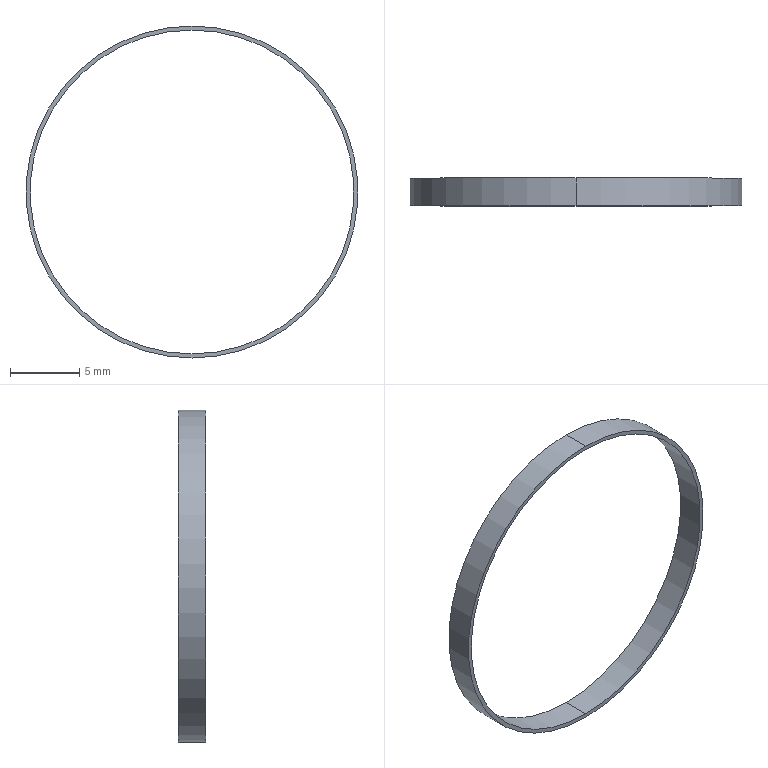Part | SolidWorks | features BaseBody 1 | 1 solid | 6 faces | box 24 x 2 x 24 mm | volume 44.673 mm3 | cylinder 4 | plane 2 | commonest cylinder face diameters 23.4 x2 24 x2
STEP:
#1=CARTESIAN_POINT('',(0.,-1.,12.));
#2=VERTEX_POINT('',#1);
#3=CARTESIAN_POINT('',(0.,-1.,-12.));
#4=VERTEX_POINT('',#3);
#5=CARTESIAN_POINT('',(0.,-1.,0.));
#6=DIRECTION('',(0.,1.,0.));
#7=DIRECTION('',(0.,0.,1.));
#8=AXIS2_PLACEMENT_3D('',#5,#6,#7);
#9=CIRCLE('',#8,12.);
#10=EDGE_CURVE('',#2,#4,#9,.T.);
#11=ORIENTED_EDGE('',*,*,#10,.T.);
#12=CARTESIAN_POINT('',(0.,1.,-12.));
#13=VERTEX_POINT('',#12);
#14=CARTESIAN_POINT('',(0.,-1.,-12.));
#15=DIRECTION('',(0.,1.,0.));
#16=VECTOR('',#15,1000.);
#17=LINE('',#14,#16);
#18=EDGE_CURVE('',#4,#13,#17,.T.);
#19=ORIENTED_EDGE('',*,*,#18,.T.);
#20=CARTESIAN_POINT('',(0.,1.,12.));
#21=VERTEX_POINT('',#20);
#22=CARTESIAN_POINT('',(0.,1.,0.));
#23=DIRECTION('',(0.,-1.,0.));
#24=DIRECTION('',(0.,0.,1.));
#25=AXIS2_PLACEMENT_3D('',#22,#23,#24);
#26=CIRCLE('',#25,12.);
#27=EDGE_CURVE('',#13,#21,#26,.T.);
#28=ORIENTED_EDGE('',*,*,#27,.T.);
#29=CARTESIAN_POINT('',(0.,-1.,12.));
#30=DIRECTION('',(0.,1.,0.));
#31=VECTOR('',#30,1000.);
#32=LINE('',#29,#31);
#33=EDGE_CURVE('',#2,#21,#32,.T.);
#34=ORIENTED_EDGE('',*,*,#33,.F.);
#35=EDGE_LOOP('',(#11,#19,#28,#34));
#36=FACE_OUTER_BOUND('',#35,.T.);
#37=CARTESIAN_POINT('',(0.,-1.,0.));
#38=DIRECTION('',(0.,1.,0.));
#39=DIRECTION('',(0.,0.,1.));
#40=AXIS2_PLACEMENT_3D('',#37,#38,#39);
#41=CYLINDRICAL_SURFACE('',#40,12.);
#42=ADVANCED_FACE('',(#36),#41,.T.);
#43=CARTESIAN_POINT('',(0.,-1.,11.7));
#44=VERTEX_POINT('',#43);
#45=CARTESIAN_POINT('',(0.,-1.,-11.7));
#46=VERTEX_POINT('',#45);
#47=CARTESIAN_POINT('',(0.,-1.,0.));
#48=DIRECTION('',(0.,-1.,0.));
#49=DIRECTION('',(0.,0.,1.));
#50=AXIS2_PLACEMENT_3D('',#47,#48,#49);
#51=CIRCLE('',#50,11.7);
#52=EDGE_CURVE('',#44,#46,#51,.T.);
#53=ORIENTED_EDGE('',*,*,#52,.T.);
#54=CARTESIAN_POINT('',(0.,1.,-11.7));
#55=VERTEX_POINT('',#54);
#56=CARTESIAN_POINT('',(0.,-2.,-11.7));
#57=DIRECTION('',(0.,1.,0.));
#58=VECTOR('',#57,1000.);
#59=LINE('',#56,#58);
#60=EDGE_CURVE('',#46,#55,#59,.T.);
#61=ORIENTED_EDGE('',*,*,#60,.T.);
#62=CARTESIAN_POINT('',(0.,1.,11.7));
#63=VERTEX_POINT('',#62);
#64=CARTESIAN_POINT('',(0.,1.,0.));
#65=DIRECTION('',(0.,-1.,0.));
#66=DIRECTION('',(0.,0.,1.));
#67=AXIS2_PLACEMENT_3D('',#64,#65,#66);
#68=CIRCLE('',#67,11.7);
#69=EDGE_CURVE('',#63,#55,#68,.T.);
#70=ORIENTED_EDGE('',*,*,#69,.F.);
#71=CARTESIAN_POINT('',(0.,-2.,11.7));
#72=DIRECTION('',(0.,1.,0.));
#73=VECTOR('',#72,1000.);
#74=LINE('',#71,#73);
#75=EDGE_CURVE('',#44,#63,#74,.T.);
#76=ORIENTED_EDGE('',*,*,#75,.F.);
#77=EDGE_LOOP('',(#53,#61,#70,#76));
#78=FACE_OUTER_BOUND('',#77,.T.);
#79=CARTESIAN_POINT('',(0.,-2.,0.));
#80=DIRECTION('',(0.,1.,0.));
#81=DIRECTION('',(0.,0.,1.));
#82=AXIS2_PLACEMENT_3D('',#79,#80,#81);
#83=CYLINDRICAL_SURFACE('',#82,11.7);
#84=ADVANCED_FACE('',(#78),#83,.F.);
#85=ORIENTED_EDGE('',*,*,#18,.F.);
#86=CARTESIAN_POINT('',(0.,-1.,0.));
#87=DIRECTION('',(0.,1.,0.));
#88=DIRECTION('',(0.,0.,1.));
#89=AXIS2_PLACEMENT_3D('',#86,#87,#88);
#90=CIRCLE('',#89,12.);
#91=EDGE_CURVE('',#4,#2,#90,.T.);
#92=ORIENTED_EDGE('',*,*,#91,.T.);
#93=ORIENTED_EDGE('',*,*,#33,.T.);
#94=CARTESIAN_POINT('',(0.,1.,0.));
#95=DIRECTION('',(0.,-1.,0.));
#96=DIRECTION('',(0.,0.,1.));
#97=AXIS2_PLACEMENT_3D('',#94,#95,#96);
#98=CIRCLE('',#97,12.);
#99=EDGE_CURVE('',#21,#13,#98,.T.);
#100=ORIENTED_EDGE('',*,*,#99,.T.);
#101=EDGE_LOOP('',(#85,#92,#93,#100));
#102=FACE_OUTER_BOUND('',#101,.T.);
#103=CARTESIAN_POINT('',(0.,-1.,0.));
#104=DIRECTION('',(0.,1.,0.));
#105=DIRECTION('',(0.,0.,1.));
#106=AXIS2_PLACEMENT_3D('',#103,#104,#105);
#107=CYLINDRICAL_SURFACE('',#106,12.);
#108=ADVANCED_FACE('',(#102),#107,.T.);
#109=ORIENTED_EDGE('',*,*,#52,.F.);
#110=CARTESIAN_POINT('',(0.,-1.,0.));
#111=DIRECTION('',(0.,-1.,0.));
#112=DIRECTION('',(0.,0.,1.));
#113=AXIS2_PLACEMENT_3D('',#110,#111,#112);
#114=CIRCLE('',#113,11.7);
#115=EDGE_CURVE('',#46,#44,#114,.T.);
#116=ORIENTED_EDGE('',*,*,#115,.F.);
#117=EDGE_LOOP('',(#109,#116));
#118=FACE_BOUND('',#117,.T.);
#119=ORIENTED_EDGE('',*,*,#10,.F.);
#120=ORIENTED_EDGE('',*,*,#91,.F.);
#121=EDGE_LOOP('',(#119,#120));
#122=FACE_OUTER_BOUND('',#121,.T.);
#123=CARTESIAN_POINT('',(0.,-1.,0.));
#124=DIRECTION('',(0.,1.,0.));
#125=DIRECTION('',(0.,0.,1.));
#126=AXIS2_PLACEMENT_3D('',#123,#124,#125);
#127=PLANE('',#126);
#128=ADVANCED_FACE('',(#118,#122),#127,.F.);
#129=ORIENTED_EDGE('',*,*,#69,.T.);
#130=CARTESIAN_POINT('',(0.,1.,0.));
#131=DIRECTION('',(0.,-1.,0.));
#132=DIRECTION('',(0.,0.,1.));
#133=AXIS2_PLACEMENT_3D('',#130,#131,#132);
#134=CIRCLE('',#133,11.7);
#135=EDGE_CURVE('',#55,#63,#134,.T.);
#136=ORIENTED_EDGE('',*,*,#135,.T.);
#137=EDGE_LOOP('',(#129,#136));
#138=FACE_BOUND('',#137,.T.);
#139=ORIENTED_EDGE('',*,*,#99,.F.);
#140=ORIENTED_EDGE('',*,*,#27,.F.);
#141=EDGE_LOOP('',(#139,#140));
#142=FACE_OUTER_BOUND('',#141,.T.);
#143=CARTESIAN_POINT('',(0.,1.,0.));
#144=DIRECTION('',(0.,1.,0.));
#145=DIRECTION('',(0.,0.,1.));
#146=AXIS2_PLACEMENT_3D('',#143,#144,#145);
#147=PLANE('',#146);
#148=ADVANCED_FACE('',(#138,#142),#147,.T.);
#149=ORIENTED_EDGE('',*,*,#60,.F.);
#150=ORIENTED_EDGE('',*,*,#115,.T.);
#151=ORIENTED_EDGE('',*,*,#75,.T.);
#152=ORIENTED_EDGE('',*,*,#135,.F.);
#153=EDGE_LOOP('',(#149,#150,#151,#152));
#154=FACE_OUTER_BOUND('',#153,.T.);
#155=CARTESIAN_POINT('',(0.,-2.,0.));
#156=DIRECTION('',(0.,1.,0.));
#157=DIRECTION('',(0.,0.,1.));
#158=AXIS2_PLACEMENT_3D('',#155,#156,#157);
#159=CYLINDRICAL_SURFACE('',#158,11.7);
#160=ADVANCED_FACE('',(#154),#159,.F.);
#161=CLOSED_SHELL('',(#42,#84,#108,#128,#148,#160));
#162=MANIFOLD_SOLID_BREP('',#161);
#163=CARTESIAN_POINT('',(0.,0.,0.));
#164=DIRECTION('',(0.,0.,1.));
#165=DIRECTION('',(1.,0.,0.));
#166=AXIS2_PLACEMENT_3D('',#163,#164,#165);
#167=(LENGTH_UNIT()NAMED_UNIT(*)SI_UNIT(.MILLI.,.METRE.));
#168=UNCERTAINTY_MEASURE_WITH_UNIT(LENGTH_MEASURE(0.00001),#167,'','');
#169=(NAMED_UNIT(*)PLANE_ANGLE_UNIT()SI_UNIT($,.RADIAN.));
#170=(NAMED_UNIT(*)SI_UNIT($,.STERADIAN.)SOLID_ANGLE_UNIT());
#171=(GEOMETRIC_REPRESENTATION_CONTEXT(3)GLOBAL_UNCERTAINTY_ASSIGNED_CONTEXT((#168))GLOBAL_UNIT_ASSIGNED_CONTEXT((#167,#169,#170))REPRESENTATION_CONTEXT('',''));
#172=ADVANCED_BREP_SHAPE_REPRESENTATION('',(#162,#166),#171);